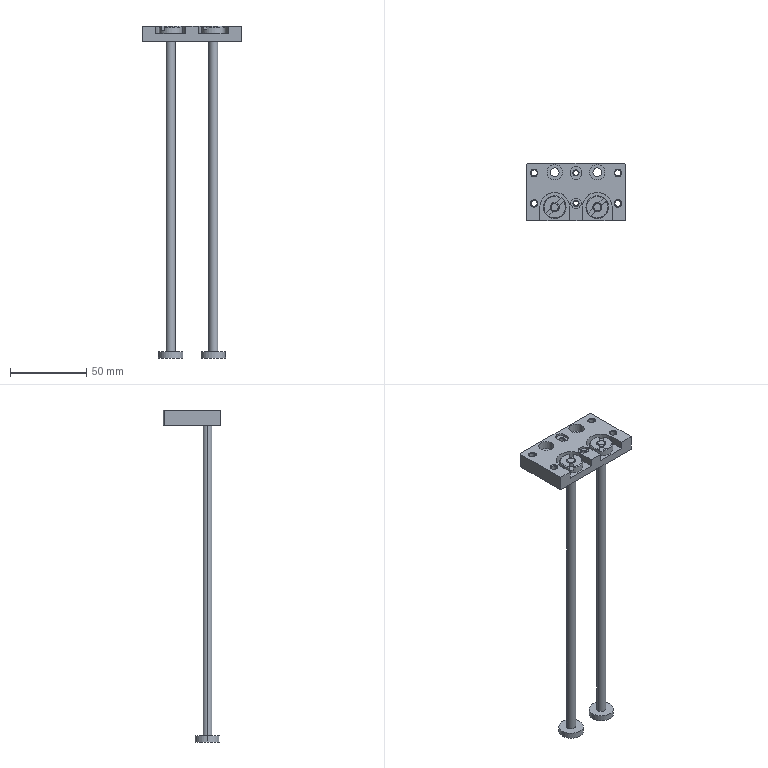Part | STEP file | 1 solid | 134 faces | box 65.6 x 38 x 218 mm | volume 33803 mm3 | cylinder 51 | plane 45 | cone 38 | commonest cylinder face diameters 6 x14 4 x8 3.2 x4 5.7 x4 7 x4 10 x4